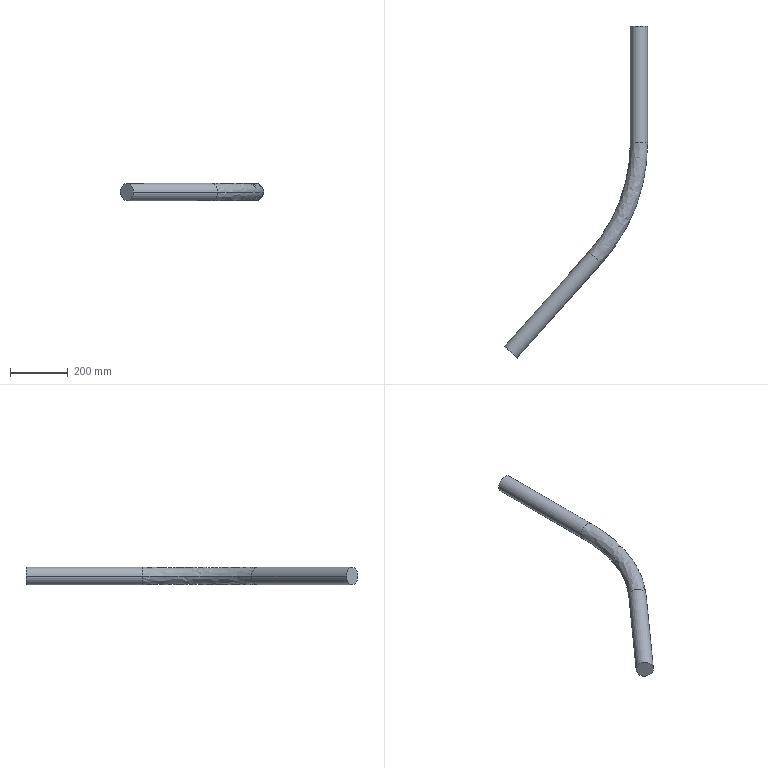Part | STEP file | 750038469 | 1 solid | 8 faces | box 497.894 x 1154 x 60 mm | volume 3628627 mm3 | cylinder 4 | spline 2 | plane 2 | commonest cylinder face diameters 60 x4
STEP:
#1=CARTESIAN_POINT('',(425.771,309.142,0.));
#2=VERTEX_POINT('',#1);
#3=CARTESIAN_POINT('',(380.984,349.067,0.));
#4=VERTEX_POINT('',#3);
#5=CARTESIAN_POINT('',(403.377,329.104,0.));
#6=DIRECTION('',(-0.6654,-0.7465,0.));
#7=DIRECTION('',(0.7465,-0.6654,0.));
#8=AXIS2_PLACEMENT_3D('',#5,#6,#7);
#9=CIRCLE('',#8,30.);
#10=EDGE_CURVE('',#2,#4,#9,.T.);
#11=ORIENTED_EDGE('',*,*,#10,.T.);
#12=CARTESIAN_POINT('',(87.606,19.963,0.));
#13=VERTEX_POINT('',#12);
#14=CARTESIAN_POINT('',(380.984,349.067,0.));
#15=DIRECTION('',(-0.6654,-0.7465,0.));
#16=VECTOR('',#15,1000.);
#17=LINE('',#14,#16);
#18=EDGE_CURVE('',#4,#13,#17,.T.);
#19=ORIENTED_EDGE('',*,*,#18,.T.);
#20=CARTESIAN_POINT('',(132.394,-19.963,0.));
#21=VERTEX_POINT('',#20);
#22=CARTESIAN_POINT('',(110.,0.,0.));
#23=DIRECTION('',(0.6654,0.7465,0.));
#24=DIRECTION('',(0.7465,-0.6654,0.));
#25=AXIS2_PLACEMENT_3D('',#22,#23,#24);
#26=CIRCLE('',#25,30.);
#27=EDGE_CURVE('',#13,#21,#26,.T.);
#28=ORIENTED_EDGE('',*,*,#27,.T.);
#29=CARTESIAN_POINT('',(425.771,309.142,0.));
#30=DIRECTION('',(-0.6654,-0.7465,0.));
#31=VECTOR('',#30,1000.);
#32=LINE('',#29,#31);
#33=EDGE_CURVE('',#2,#21,#32,.T.);
#34=ORIENTED_EDGE('',*,*,#33,.F.);
#35=EDGE_LOOP('',(#11,#19,#28,#34));
#36=FACE_OUTER_BOUND('',#35,.T.);
#37=CARTESIAN_POINT('',(403.377,329.104,0.));
#38=DIRECTION('',(-0.6654,-0.7465,0.));
#39=DIRECTION('',(0.7465,-0.6654,0.));
#40=AXIS2_PLACEMENT_3D('',#37,#38,#39);
#41=CYLINDRICAL_SURFACE('',#40,30.);
#42=ADVANCED_FACE('',(#36),#41,.T.);
#43=CARTESIAN_POINT('',(403.377,329.104,0.));
#44=DIRECTION('',(-0.6654,-0.7465,0.));
#45=DIRECTION('',(0.7465,-0.6654,0.));
#46=AXIS2_PLACEMENT_3D('',#43,#44,#45);
#47=CIRCLE('',#46,30.);
#48=EDGE_CURVE('',#4,#2,#47,.T.);
#49=ORIENTED_EDGE('',*,*,#48,.F.);
#50=CARTESIAN_POINT('',(525.5,728.361,0.));
#51=VERTEX_POINT('',#50);
#52=CARTESIAN_POINT('',(-44.5,728.361,0.));
#53=DIRECTION('',(0.,0.,1.));
#54=DIRECTION('',(1.,0.,0.));
#55=AXIS2_PLACEMENT_3D('',#52,#53,#54);
#56=CIRCLE('',#55,570.);
#57=EDGE_CURVE('',#4,#51,#56,.T.);
#58=ORIENTED_EDGE('',*,*,#57,.T.);
#59=CARTESIAN_POINT('',(585.5,728.361,0.));
#60=VERTEX_POINT('',#59);
#61=CARTESIAN_POINT('',(555.5,728.361,0.));
#62=DIRECTION('',(0.,-1.,0.));
#63=DIRECTION('',(1.,0.,0.));
#64=AXIS2_PLACEMENT_3D('',#61,#62,#63);
#65=CIRCLE('',#64,30.);
#66=EDGE_CURVE('',#51,#60,#65,.T.);
#67=ORIENTED_EDGE('',*,*,#66,.T.);
#68=CARTESIAN_POINT('',(-44.5,728.361,0.));
#69=DIRECTION('',(0.,0.,1.));
#70=DIRECTION('',(1.,0.,0.));
#71=AXIS2_PLACEMENT_3D('',#68,#69,#70);
#72=CIRCLE('',#71,630.);
#73=EDGE_CURVE('',#2,#60,#72,.T.);
#74=ORIENTED_EDGE('',*,*,#73,.F.);
#75=EDGE_LOOP('',(#49,#58,#67,#74));
#76=FACE_OUTER_BOUND('',#75,.T.);
#77=CARTESIAN_POINT('',(425.771,309.142,0.));
#78=CARTESIAN_POINT('',(529.825,425.867,0.));
#79=CARTESIAN_POINT('',(585.5,571.99,0.));
#80=CARTESIAN_POINT('',(585.5,728.361,0.));
#81=CARTESIAN_POINT('',(425.771,309.142,-60.));
#82=CARTESIAN_POINT('',(529.825,425.867,-60.));
#83=CARTESIAN_POINT('',(585.5,571.99,-60.));
#84=CARTESIAN_POINT('',(585.5,728.361,-60.));
#85=CARTESIAN_POINT('',(380.984,349.067,-60.));
#86=CARTESIAN_POINT('',(475.127,454.676,-60.));
#87=CARTESIAN_POINT('',(525.5,586.883,-60.));
#88=CARTESIAN_POINT('',(525.5,728.361,-60.));
#89=CARTESIAN_POINT('',(380.984,349.067,0.));
#90=CARTESIAN_POINT('',(475.127,454.676,0.));
#91=CARTESIAN_POINT('',(525.5,586.883,0.));
#92=CARTESIAN_POINT('',(525.5,728.361,0.));
#93=(BOUNDED_SURFACE()B_SPLINE_SURFACE(3,3,((#77,#78,#79,#80),(#81,#82,#83,#84),(#85,#86,#87,#88),(#89,#90,#91,#92)),.UNSPECIFIED.,.F.,.F.,.F.)B_SPLINE_SURFACE_WITH_KNOTS((4,4),(4,4),(0.,1.),(0.,1.),.UNSPECIFIED.)GEOMETRIC_REPRESENTATION_ITEM()RATIONAL_B_SPLINE_SURFACE(((1.,0.9563,0.9563,1.),(0.3333,0.3188,0.3188,0.3333),(0.3333,0.3188,0.3188,0.3333),(1.,0.9563,0.9563,1.)))REPRESENTATION_ITEM('')SURFACE());
#94=ADVANCED_FACE('',(#76),#93,.T.);
#95=CARTESIAN_POINT('',(555.5,728.361,0.));
#96=DIRECTION('',(0.,-1.,0.));
#97=DIRECTION('',(1.,0.,0.));
#98=AXIS2_PLACEMENT_3D('',#95,#96,#97);
#99=CIRCLE('',#98,30.);
#100=EDGE_CURVE('',#60,#51,#99,.T.);
#101=ORIENTED_EDGE('',*,*,#100,.F.);
#102=CARTESIAN_POINT('',(585.5,1134.,0.));
#103=VERTEX_POINT('',#102);
#104=CARTESIAN_POINT('',(585.5,728.361,0.));
#105=DIRECTION('',(0.,1.,0.));
#106=VECTOR('',#105,1000.);
#107=LINE('',#104,#106);
#108=EDGE_CURVE('',#60,#103,#107,.T.);
#109=ORIENTED_EDGE('',*,*,#108,.T.);
#110=CARTESIAN_POINT('',(525.5,1134.,0.));
#111=VERTEX_POINT('',#110);
#112=CARTESIAN_POINT('',(555.5,1134.,0.));
#113=DIRECTION('',(0.,-1.,0.));
#114=DIRECTION('',(-1.,0.,0.));
#115=AXIS2_PLACEMENT_3D('',#112,#113,#114);
#116=CIRCLE('',#115,30.);
#117=EDGE_CURVE('',#103,#111,#116,.T.);
#118=ORIENTED_EDGE('',*,*,#117,.T.);
#119=CARTESIAN_POINT('',(525.5,728.361,0.));
#120=DIRECTION('',(0.,1.,0.));
#121=VECTOR('',#120,1000.);
#122=LINE('',#119,#121);
#123=EDGE_CURVE('',#51,#111,#122,.T.);
#124=ORIENTED_EDGE('',*,*,#123,.F.);
#125=EDGE_LOOP('',(#101,#109,#118,#124));
#126=FACE_OUTER_BOUND('',#125,.T.);
#127=CARTESIAN_POINT('',(555.5,728.361,0.));
#128=DIRECTION('',(0.,1.,0.));
#129=DIRECTION('',(-1.,0.,0.));
#130=AXIS2_PLACEMENT_3D('',#127,#128,#129);
#131=CYLINDRICAL_SURFACE('',#130,30.);
#132=ADVANCED_FACE('',(#126),#131,.T.);
#133=ORIENTED_EDGE('',*,*,#18,.F.);
#134=ORIENTED_EDGE('',*,*,#48,.T.);
#135=ORIENTED_EDGE('',*,*,#33,.T.);
#136=CARTESIAN_POINT('',(110.,0.,0.));
#137=DIRECTION('',(0.6654,0.7465,0.));
#138=DIRECTION('',(0.7465,-0.6654,0.));
#139=AXIS2_PLACEMENT_3D('',#136,#137,#138);
#140=CIRCLE('',#139,30.);
#141=EDGE_CURVE('',#21,#13,#140,.T.);
#142=ORIENTED_EDGE('',*,*,#141,.T.);
#143=EDGE_LOOP('',(#133,#134,#135,#142));
#144=FACE_OUTER_BOUND('',#143,.T.);
#145=CARTESIAN_POINT('',(403.377,329.104,0.));
#146=DIRECTION('',(-0.6654,-0.7465,0.));
#147=DIRECTION('',(0.7465,-0.6654,0.));
#148=AXIS2_PLACEMENT_3D('',#145,#146,#147);
#149=CYLINDRICAL_SURFACE('',#148,30.);
#150=ADVANCED_FACE('',(#144),#149,.T.);
#151=ORIENTED_EDGE('',*,*,#141,.F.);
#152=ORIENTED_EDGE('',*,*,#27,.F.);
#153=EDGE_LOOP('',(#151,#152));
#154=FACE_OUTER_BOUND('',#153,.T.);
#155=CARTESIAN_POINT('',(110.,0.,0.));
#156=DIRECTION('',(0.6654,0.7465,0.));
#157=DIRECTION('',(-0.7465,0.6654,0.));
#158=AXIS2_PLACEMENT_3D('',#155,#156,#157);
#159=PLANE('',#158);
#160=ADVANCED_FACE('',(#154),#159,.F.);
#161=ORIENTED_EDGE('',*,*,#57,.F.);
#162=ORIENTED_EDGE('',*,*,#10,.F.);
#163=ORIENTED_EDGE('',*,*,#73,.T.);
#164=ORIENTED_EDGE('',*,*,#100,.T.);
#165=EDGE_LOOP('',(#161,#162,#163,#164));
#166=FACE_OUTER_BOUND('',#165,.T.);
#167=CARTESIAN_POINT('',(380.984,349.067,0.));
#168=CARTESIAN_POINT('',(475.127,454.676,0.));
#169=CARTESIAN_POINT('',(525.5,586.883,0.));
#170=CARTESIAN_POINT('',(525.5,728.361,0.));
#171=CARTESIAN_POINT('',(380.984,349.067,60.));
#172=CARTESIAN_POINT('',(475.127,454.676,60.));
#173=CARTESIAN_POINT('',(525.5,586.883,60.));
#174=CARTESIAN_POINT('',(525.5,728.361,60.));
#175=CARTESIAN_POINT('',(425.771,309.142,60.));
#176=CARTESIAN_POINT('',(529.825,425.867,60.));
#177=CARTESIAN_POINT('',(585.5,571.99,60.));
#178=CARTESIAN_POINT('',(585.5,728.361,60.));
#179=CARTESIAN_POINT('',(425.771,309.142,0.));
#180=CARTESIAN_POINT('',(529.825,425.867,0.));
#181=CARTESIAN_POINT('',(585.5,571.99,0.));
#182=CARTESIAN_POINT('',(585.5,728.361,0.));
#183=(BOUNDED_SURFACE()B_SPLINE_SURFACE(3,3,((#167,#168,#169,#170),(#171,#172,#173,#174),(#175,#176,#177,#178),(#179,#180,#181,#182)),.UNSPECIFIED.,.F.,.F.,.F.)B_SPLINE_SURFACE_WITH_KNOTS((4,4),(4,4),(0.,1.),(0.,1.),.UNSPECIFIED.)GEOMETRIC_REPRESENTATION_ITEM()RATIONAL_B_SPLINE_SURFACE(((1.,0.9563,0.9563,1.),(0.3333,0.3188,0.3188,0.3333),(0.3333,0.3188,0.3188,0.3333),(1.,0.9563,0.9563,1.)))REPRESENTATION_ITEM('')SURFACE());
#184=ADVANCED_FACE('',(#166),#183,.T.);
#185=ORIENTED_EDGE('',*,*,#108,.F.);
#186=ORIENTED_EDGE('',*,*,#66,.F.);
#187=ORIENTED_EDGE('',*,*,#123,.T.);
#188=CARTESIAN_POINT('',(555.5,1134.,0.));
#189=DIRECTION('',(0.,-1.,0.));
#190=DIRECTION('',(-1.,0.,0.));
#191=AXIS2_PLACEMENT_3D('',#188,#189,#190);
#192=CIRCLE('',#191,30.);
#193=EDGE_CURVE('',#111,#103,#192,.T.);
#194=ORIENTED_EDGE('',*,*,#193,.T.);
#195=EDGE_LOOP('',(#185,#186,#187,#194));
#196=FACE_OUTER_BOUND('',#195,.T.);
#197=CARTESIAN_POINT('',(555.5,728.361,0.));
#198=DIRECTION('',(0.,1.,0.));
#199=DIRECTION('',(-1.,0.,0.));
#200=AXIS2_PLACEMENT_3D('',#197,#198,#199);
#201=CYLINDRICAL_SURFACE('',#200,30.);
#202=ADVANCED_FACE('',(#196),#201,.T.);
#203=ORIENTED_EDGE('',*,*,#193,.F.);
#204=ORIENTED_EDGE('',*,*,#117,.F.);
#205=EDGE_LOOP('',(#203,#204));
#206=FACE_OUTER_BOUND('',#205,.T.);
#207=CARTESIAN_POINT('',(555.5,1134.,0.));
#208=DIRECTION('',(0.,1.,0.));
#209=DIRECTION('',(-1.,0.,0.));
#210=AXIS2_PLACEMENT_3D('',#207,#208,#209);
#211=PLANE('',#210);
#212=ADVANCED_FACE('',(#206),#211,.T.);
#213=CLOSED_SHELL('',(#42,#94,#132,#150,#160,#184,#202,#212));
#214=MANIFOLD_SOLID_BREP('',#213);
#215=CARTESIAN_POINT('',(0.,0.,0.));
#216=DIRECTION('',(0.,0.,1.));
#217=DIRECTION('',(1.,0.,0.));
#218=AXIS2_PLACEMENT_3D('',#215,#216,#217);
#219=(LENGTH_UNIT()NAMED_UNIT(*)SI_UNIT(.MILLI.,.METRE.));
#220=UNCERTAINTY_MEASURE_WITH_UNIT(LENGTH_MEASURE(0.00001),#219,'','');
#221=(NAMED_UNIT(*)PLANE_ANGLE_UNIT()SI_UNIT($,.RADIAN.));
#222=(NAMED_UNIT(*)SI_UNIT($,.STERADIAN.)SOLID_ANGLE_UNIT());
#223=(GEOMETRIC_REPRESENTATION_CONTEXT(3)GLOBAL_UNCERTAINTY_ASSIGNED_CONTEXT((#220))GLOBAL_UNIT_ASSIGNED_CONTEXT((#219,#221,#222))REPRESENTATION_CONTEXT('',''));
#224=ADVANCED_BREP_SHAPE_REPRESENTATION('',(#214,#218),#223);